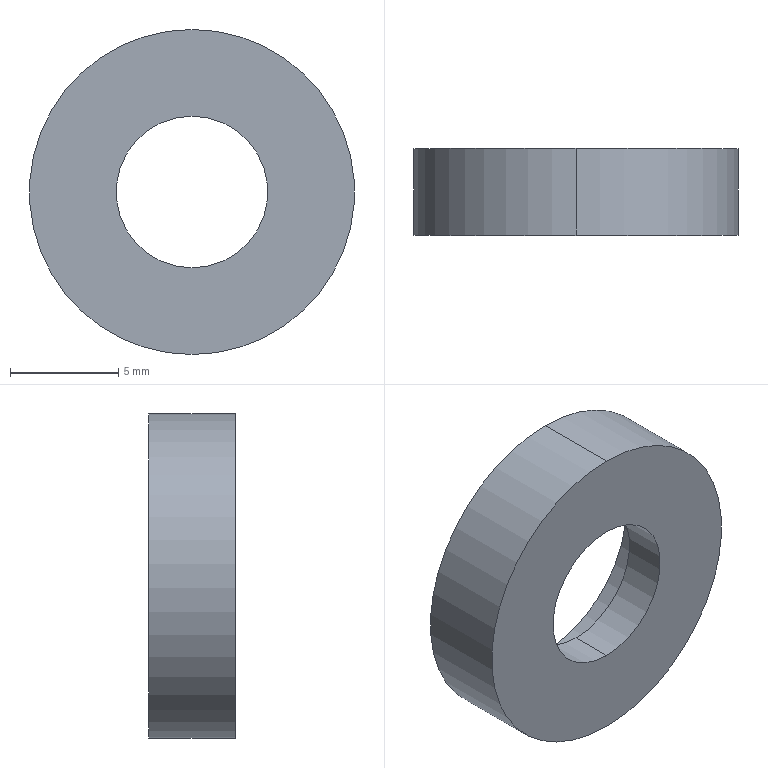Part | SolidWorks | features Revolution 1 | 1 solid | 9 faces | box 15 x 4 x 15 mm | volume 456.709 mm3 | cylinder 6 | plane 3 | commonest cylinder face diameters 7 x2 10.5 x2 15 x2
STEP:
#1=CARTESIAN_POINT('',(0.,2.,3.5));
#2=VERTEX_POINT('',#1);
#3=CARTESIAN_POINT('',(0.,2.,-3.5));
#4=VERTEX_POINT('',#3);
#5=CARTESIAN_POINT('',(0.,2.,0.));
#6=DIRECTION('',(0.,-1.,0.));
#7=DIRECTION('',(0.,0.,-1.));
#8=AXIS2_PLACEMENT_3D('',#5,#6,#7);
#9=CIRCLE('',#8,3.5);
#10=EDGE_CURVE('',#2,#4,#9,.T.);
#11=ORIENTED_EDGE('',*,*,#10,.F.);
#12=CARTESIAN_POINT('',(0.,0.,3.5));
#13=VERTEX_POINT('',#12);
#14=CARTESIAN_POINT('',(0.,0.,3.5));
#15=DIRECTION('',(0.,-1.,0.));
#16=VECTOR('',#15,1000.);
#17=LINE('',#14,#16);
#18=EDGE_CURVE('',#2,#13,#17,.T.);
#19=ORIENTED_EDGE('',*,*,#18,.T.);
#20=CARTESIAN_POINT('',(0.,0.,-3.5));
#21=VERTEX_POINT('',#20);
#22=CARTESIAN_POINT('',(0.,0.,0.));
#23=DIRECTION('',(0.,-1.,0.));
#24=DIRECTION('',(0.,0.,-1.));
#25=AXIS2_PLACEMENT_3D('',#22,#23,#24);
#26=CIRCLE('',#25,3.5);
#27=EDGE_CURVE('',#13,#21,#26,.T.);
#28=ORIENTED_EDGE('',*,*,#27,.T.);
#29=CARTESIAN_POINT('',(0.,0.,-3.5));
#30=DIRECTION('',(0.,-1.,0.));
#31=VECTOR('',#30,1000.);
#32=LINE('',#29,#31);
#33=EDGE_CURVE('',#4,#21,#32,.T.);
#34=ORIENTED_EDGE('',*,*,#33,.F.);
#35=EDGE_LOOP('',(#11,#19,#28,#34));
#36=FACE_OUTER_BOUND('',#35,.T.);
#37=CARTESIAN_POINT('',(0.,0.,0.));
#38=DIRECTION('',(0.,-1.,0.));
#39=DIRECTION('',(0.,0.,-1.));
#40=AXIS2_PLACEMENT_3D('',#37,#38,#39);
#41=CYLINDRICAL_SURFACE('',#40,3.5);
#42=ADVANCED_FACE('',(#36),#41,.F.);
#43=CARTESIAN_POINT('',(0.,4.,5.25));
#44=VERTEX_POINT('',#43);
#45=CARTESIAN_POINT('',(0.,4.,-5.25));
#46=VERTEX_POINT('',#45);
#47=CARTESIAN_POINT('',(0.,4.,0.));
#48=DIRECTION('',(0.,-1.,0.));
#49=DIRECTION('',(0.,0.,-1.));
#50=AXIS2_PLACEMENT_3D('',#47,#48,#49);
#51=CIRCLE('',#50,5.25);
#52=EDGE_CURVE('',#44,#46,#51,.T.);
#53=ORIENTED_EDGE('',*,*,#52,.F.);
#54=CARTESIAN_POINT('',(0.,2.,5.25));
#55=VERTEX_POINT('',#54);
#56=CARTESIAN_POINT('',(0.,0.,5.25));
#57=DIRECTION('',(0.,-1.,0.));
#58=VECTOR('',#57,1000.);
#59=LINE('',#56,#58);
#60=EDGE_CURVE('',#44,#55,#59,.T.);
#61=ORIENTED_EDGE('',*,*,#60,.T.);
#62=CARTESIAN_POINT('',(0.,2.,-5.25));
#63=VERTEX_POINT('',#62);
#64=CARTESIAN_POINT('',(0.,2.,0.));
#65=DIRECTION('',(0.,-1.,0.));
#66=DIRECTION('',(0.,0.,-1.));
#67=AXIS2_PLACEMENT_3D('',#64,#65,#66);
#68=CIRCLE('',#67,5.25);
#69=EDGE_CURVE('',#55,#63,#68,.T.);
#70=ORIENTED_EDGE('',*,*,#69,.T.);
#71=CARTESIAN_POINT('',(0.,0.,-5.25));
#72=DIRECTION('',(0.,-1.,0.));
#73=VECTOR('',#72,1000.);
#74=LINE('',#71,#73);
#75=EDGE_CURVE('',#46,#63,#74,.T.);
#76=ORIENTED_EDGE('',*,*,#75,.F.);
#77=EDGE_LOOP('',(#53,#61,#70,#76));
#78=FACE_OUTER_BOUND('',#77,.T.);
#79=CARTESIAN_POINT('',(0.,0.,0.));
#80=DIRECTION('',(0.,-1.,0.));
#81=DIRECTION('',(0.,0.,-1.));
#82=AXIS2_PLACEMENT_3D('',#79,#80,#81);
#83=CYLINDRICAL_SURFACE('',#82,5.25);
#84=ADVANCED_FACE('',(#78),#83,.F.);
#85=CARTESIAN_POINT('',(0.,4.,-7.5));
#86=VERTEX_POINT('',#85);
#87=CARTESIAN_POINT('',(0.,4.,7.5));
#88=VERTEX_POINT('',#87);
#89=CARTESIAN_POINT('',(0.,4.,0.));
#90=DIRECTION('',(0.,-1.,0.));
#91=DIRECTION('',(0.,0.,-1.));
#92=AXIS2_PLACEMENT_3D('',#89,#90,#91);
#93=CIRCLE('',#92,7.5);
#94=EDGE_CURVE('',#86,#88,#93,.T.);
#95=ORIENTED_EDGE('',*,*,#94,.T.);
#96=CARTESIAN_POINT('',(0.,0.,7.5));
#97=VERTEX_POINT('',#96);
#98=CARTESIAN_POINT('',(0.,0.,7.5));
#99=DIRECTION('',(0.,-1.,0.));
#100=VECTOR('',#99,1000.);
#101=LINE('',#98,#100);
#102=EDGE_CURVE('',#88,#97,#101,.T.);
#103=ORIENTED_EDGE('',*,*,#102,.T.);
#104=CARTESIAN_POINT('',(0.,0.,-7.5));
#105=VERTEX_POINT('',#104);
#106=CARTESIAN_POINT('',(0.,0.,0.));
#107=DIRECTION('',(0.,-1.,0.));
#108=DIRECTION('',(0.,0.,-1.));
#109=AXIS2_PLACEMENT_3D('',#106,#107,#108);
#110=CIRCLE('',#109,7.5);
#111=EDGE_CURVE('',#105,#97,#110,.T.);
#112=ORIENTED_EDGE('',*,*,#111,.F.);
#113=CARTESIAN_POINT('',(0.,0.,-7.5));
#114=DIRECTION('',(0.,-1.,0.));
#115=VECTOR('',#114,1000.);
#116=LINE('',#113,#115);
#117=EDGE_CURVE('',#86,#105,#116,.T.);
#118=ORIENTED_EDGE('',*,*,#117,.F.);
#119=EDGE_LOOP('',(#95,#103,#112,#118));
#120=FACE_OUTER_BOUND('',#119,.T.);
#121=CARTESIAN_POINT('',(0.,0.,0.));
#122=DIRECTION('',(0.,-1.,0.));
#123=DIRECTION('',(0.,0.,-1.));
#124=AXIS2_PLACEMENT_3D('',#121,#122,#123);
#125=CYLINDRICAL_SURFACE('',#124,7.5);
#126=ADVANCED_FACE('',(#120),#125,.T.);
#127=ORIENTED_EDGE('',*,*,#102,.F.);
#128=CARTESIAN_POINT('',(0.,4.,0.));
#129=DIRECTION('',(0.,-1.,0.));
#130=DIRECTION('',(0.,0.,-1.));
#131=AXIS2_PLACEMENT_3D('',#128,#129,#130);
#132=CIRCLE('',#131,7.5);
#133=EDGE_CURVE('',#88,#86,#132,.T.);
#134=ORIENTED_EDGE('',*,*,#133,.T.);
#135=ORIENTED_EDGE('',*,*,#117,.T.);
#136=CARTESIAN_POINT('',(0.,0.,0.));
#137=DIRECTION('',(0.,-1.,0.));
#138=DIRECTION('',(0.,0.,-1.));
#139=AXIS2_PLACEMENT_3D('',#136,#137,#138);
#140=CIRCLE('',#139,7.5);
#141=EDGE_CURVE('',#97,#105,#140,.T.);
#142=ORIENTED_EDGE('',*,*,#141,.F.);
#143=EDGE_LOOP('',(#127,#134,#135,#142));
#144=FACE_OUTER_BOUND('',#143,.T.);
#145=CARTESIAN_POINT('',(0.,0.,0.));
#146=DIRECTION('',(0.,-1.,0.));
#147=DIRECTION('',(0.,0.,-1.));
#148=AXIS2_PLACEMENT_3D('',#145,#146,#147);
#149=CYLINDRICAL_SURFACE('',#148,7.5);
#150=ADVANCED_FACE('',(#144),#149,.T.);
#151=ORIENTED_EDGE('',*,*,#94,.F.);
#152=ORIENTED_EDGE('',*,*,#133,.F.);
#153=EDGE_LOOP('',(#151,#152));
#154=FACE_OUTER_BOUND('',#153,.T.);
#155=CARTESIAN_POINT('',(0.,4.,0.));
#156=DIRECTION('',(0.,-1.,0.));
#157=DIRECTION('',(0.,0.,-1.));
#158=AXIS2_PLACEMENT_3D('',#155,#156,#157);
#159=CIRCLE('',#158,5.25);
#160=EDGE_CURVE('',#46,#44,#159,.T.);
#161=ORIENTED_EDGE('',*,*,#160,.T.);
#162=ORIENTED_EDGE('',*,*,#52,.T.);
#163=EDGE_LOOP('',(#161,#162));
#164=FACE_BOUND('',#163,.T.);
#165=CARTESIAN_POINT('',(-7.5,4.,0.));
#166=DIRECTION('',(0.,-1.,0.));
#167=DIRECTION('',(0.,0.,-1.));
#168=AXIS2_PLACEMENT_3D('',#165,#166,#167);
#169=PLANE('',#168);
#170=ADVANCED_FACE('',(#154,#164),#169,.F.);
#171=ORIENTED_EDGE('',*,*,#60,.F.);
#172=ORIENTED_EDGE('',*,*,#160,.F.);
#173=ORIENTED_EDGE('',*,*,#75,.T.);
#174=CARTESIAN_POINT('',(0.,2.,0.));
#175=DIRECTION('',(0.,-1.,0.));
#176=DIRECTION('',(0.,0.,-1.));
#177=AXIS2_PLACEMENT_3D('',#174,#175,#176);
#178=CIRCLE('',#177,5.25);
#179=EDGE_CURVE('',#63,#55,#178,.T.);
#180=ORIENTED_EDGE('',*,*,#179,.T.);
#181=EDGE_LOOP('',(#171,#172,#173,#180));
#182=FACE_OUTER_BOUND('',#181,.T.);
#183=CARTESIAN_POINT('',(0.,0.,0.));
#184=DIRECTION('',(0.,-1.,0.));
#185=DIRECTION('',(0.,0.,-1.));
#186=AXIS2_PLACEMENT_3D('',#183,#184,#185);
#187=CYLINDRICAL_SURFACE('',#186,5.25);
#188=ADVANCED_FACE('',(#182),#187,.F.);
#189=ORIENTED_EDGE('',*,*,#179,.F.);
#190=ORIENTED_EDGE('',*,*,#69,.F.);
#191=EDGE_LOOP('',(#189,#190));
#192=FACE_OUTER_BOUND('',#191,.T.);
#193=CARTESIAN_POINT('',(0.,2.,0.));
#194=DIRECTION('',(0.,-1.,0.));
#195=DIRECTION('',(0.,0.,-1.));
#196=AXIS2_PLACEMENT_3D('',#193,#194,#195);
#197=CIRCLE('',#196,3.5);
#198=EDGE_CURVE('',#4,#2,#197,.T.);
#199=ORIENTED_EDGE('',*,*,#198,.T.);
#200=ORIENTED_EDGE('',*,*,#10,.T.);
#201=EDGE_LOOP('',(#199,#200));
#202=FACE_BOUND('',#201,.T.);
#203=CARTESIAN_POINT('',(-5.25,2.,0.));
#204=DIRECTION('',(0.,-1.,0.));
#205=DIRECTION('',(0.,0.,-1.));
#206=AXIS2_PLACEMENT_3D('',#203,#204,#205);
#207=PLANE('',#206);
#208=ADVANCED_FACE('',(#192,#202),#207,.F.);
#209=ORIENTED_EDGE('',*,*,#18,.F.);
#210=ORIENTED_EDGE('',*,*,#198,.F.);
#211=ORIENTED_EDGE('',*,*,#33,.T.);
#212=CARTESIAN_POINT('',(0.,0.,0.));
#213=DIRECTION('',(0.,-1.,0.));
#214=DIRECTION('',(0.,0.,-1.));
#215=AXIS2_PLACEMENT_3D('',#212,#213,#214);
#216=CIRCLE('',#215,3.5);
#217=EDGE_CURVE('',#21,#13,#216,.T.);
#218=ORIENTED_EDGE('',*,*,#217,.T.);
#219=EDGE_LOOP('',(#209,#210,#211,#218));
#220=FACE_OUTER_BOUND('',#219,.T.);
#221=CARTESIAN_POINT('',(0.,0.,0.));
#222=DIRECTION('',(0.,-1.,0.));
#223=DIRECTION('',(0.,0.,-1.));
#224=AXIS2_PLACEMENT_3D('',#221,#222,#223);
#225=CYLINDRICAL_SURFACE('',#224,3.5);
#226=ADVANCED_FACE('',(#220),#225,.F.);
#227=ORIENTED_EDGE('',*,*,#217,.F.);
#228=ORIENTED_EDGE('',*,*,#27,.F.);
#229=EDGE_LOOP('',(#227,#228));
#230=FACE_BOUND('',#229,.T.);
#231=ORIENTED_EDGE('',*,*,#111,.T.);
#232=ORIENTED_EDGE('',*,*,#141,.T.);
#233=EDGE_LOOP('',(#231,#232));
#234=FACE_OUTER_BOUND('',#233,.T.);
#235=CARTESIAN_POINT('',(-3.5,0.,0.));
#236=DIRECTION('',(0.,1.,0.));
#237=DIRECTION('',(0.,0.,1.));
#238=AXIS2_PLACEMENT_3D('',#235,#236,#237);
#239=PLANE('',#238);
#240=ADVANCED_FACE('',(#230,#234),#239,.F.);
#241=CLOSED_SHELL('',(#42,#84,#126,#150,#170,#188,#208,#226,#240));
#242=MANIFOLD_SOLID_BREP('',#241);
#243=CARTESIAN_POINT('',(0.,0.,0.));
#244=DIRECTION('',(0.,0.,1.));
#245=DIRECTION('',(1.,0.,0.));
#246=AXIS2_PLACEMENT_3D('',#243,#244,#245);
#247=(LENGTH_UNIT()NAMED_UNIT(*)SI_UNIT(.MILLI.,.METRE.));
#248=UNCERTAINTY_MEASURE_WITH_UNIT(LENGTH_MEASURE(0.00001),#247,'','');
#249=(NAMED_UNIT(*)PLANE_ANGLE_UNIT()SI_UNIT($,.RADIAN.));
#250=(NAMED_UNIT(*)SI_UNIT($,.STERADIAN.)SOLID_ANGLE_UNIT());
#251=(GEOMETRIC_REPRESENTATION_CONTEXT(3)GLOBAL_UNCERTAINTY_ASSIGNED_CONTEXT((#248))GLOBAL_UNIT_ASSIGNED_CONTEXT((#247,#249,#250))REPRESENTATION_CONTEXT('',''));
#252=ADVANCED_BREP_SHAPE_REPRESENTATION('',(#242,#246),#251);